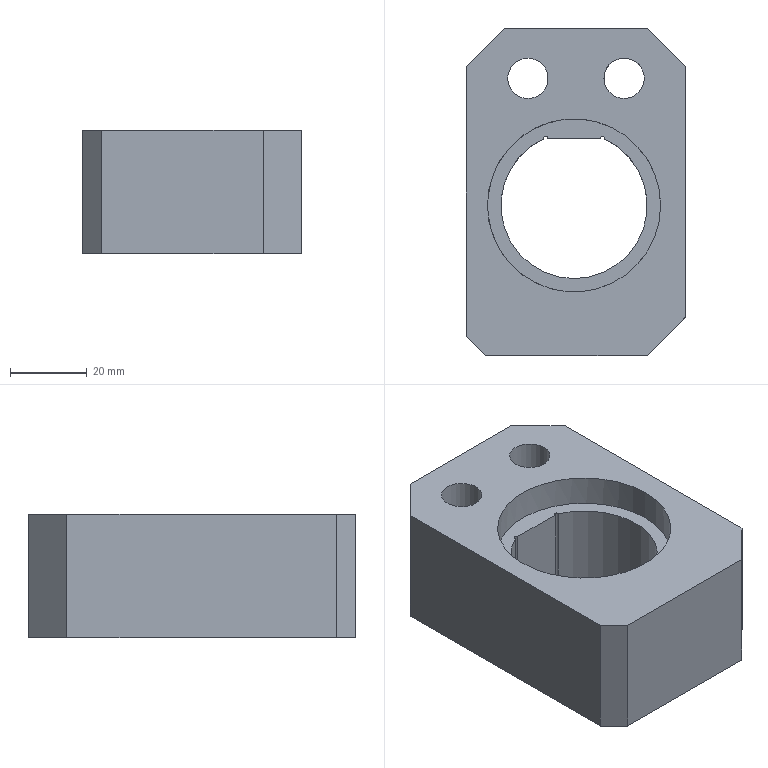Part | STEP file | lll_id3522_x_t | 1 solid | 23 faces | box 57 x 85 x 32 mm | volume 99919 mm3 | plane 14 | cylinder 9 | commonest cylinder face diameters 1 x2 10.5 x2 17 x2 38 x2 45 x1
STEP:
#1=CARTESIAN_POINT('',(3442.,57.,84.5));
#2=VERTEX_POINT('',#1);
#3=CARTESIAN_POINT('',(3419.5,57.,84.5));
#4=DIRECTION('',(0.,0.,-1.));
#5=DIRECTION('',(1.,0.,0.));
#6=AXIS2_PLACEMENT_3D('',#3,#4,#5);
#7=CIRCLE('',#6,22.5);
#8=EDGE_CURVE('',#2,#2,#7,.T.);
#9=ORIENTED_EDGE('',*,*,#8,.F.);
#10=EDGE_LOOP('',(#9));
#11=FACE_BOUND('',#10,.T.);
#12=CARTESIAN_POINT('',(3427.357,74.299,84.5));
#13=VERTEX_POINT('',#12);
#14=CARTESIAN_POINT('',(3426.399,74.5,84.5));
#15=VERTEX_POINT('',#14);
#16=CARTESIAN_POINT('',(3426.899,74.5,84.5));
#17=DIRECTION('',(0.,0.,1.));
#18=DIRECTION('',(-1.,0.,0.));
#19=AXIS2_PLACEMENT_3D('',#16,#17,#18);
#20=CIRCLE('',#19,0.5);
#21=EDGE_CURVE('',#13,#15,#20,.T.);
#22=ORIENTED_EDGE('',*,*,#21,.F.);
#23=CARTESIAN_POINT('',(3419.5,38.,84.5));
#24=VERTEX_POINT('',#23);
#25=CARTESIAN_POINT('',(3419.5,57.,84.5));
#26=DIRECTION('',(0.,0.,1.));
#27=DIRECTION('',(0.,-1.,0.));
#28=AXIS2_PLACEMENT_3D('',#25,#26,#27);
#29=CIRCLE('',#28,19.);
#30=EDGE_CURVE('',#24,#13,#29,.T.);
#31=ORIENTED_EDGE('',*,*,#30,.F.);
#32=CARTESIAN_POINT('',(3411.643,74.299,84.5));
#33=VERTEX_POINT('',#32);
#34=CARTESIAN_POINT('',(3419.5,57.,84.5));
#35=DIRECTION('',(0.,0.,1.));
#36=DIRECTION('',(0.,-1.,0.));
#37=AXIS2_PLACEMENT_3D('',#34,#35,#36);
#38=CIRCLE('',#37,19.);
#39=EDGE_CURVE('',#33,#24,#38,.T.);
#40=ORIENTED_EDGE('',*,*,#39,.F.);
#41=CARTESIAN_POINT('',(3412.601,74.5,84.5));
#42=VERTEX_POINT('',#41);
#43=CARTESIAN_POINT('',(3412.101,74.5,84.5));
#44=DIRECTION('',(0.,0.,-1.));
#45=DIRECTION('',(1.,0.,0.));
#46=AXIS2_PLACEMENT_3D('',#43,#44,#45);
#47=CIRCLE('',#46,0.5);
#48=EDGE_CURVE('',#33,#42,#47,.T.);
#49=ORIENTED_EDGE('',*,*,#48,.T.);
#50=CARTESIAN_POINT('',(3439.75,74.5,84.5));
#51=DIRECTION('',(1.,0.,0.));
#52=VECTOR('',#51,1.);
#53=LINE('',#50,#52);
#54=EDGE_CURVE('',#42,#15,#53,.T.);
#55=ORIENTED_EDGE('',*,*,#54,.T.);
#56=EDGE_LOOP('',(#22,#31,#40,#49,#55));
#57=FACE_BOUND('',#56,.T.);
#58=CARTESIAN_POINT('',(3439.75,57.,84.5));
#59=DIRECTION('',(0.,0.,-1.));
#60=DIRECTION('',(1.,0.,0.));
#61=AXIS2_PLACEMENT_3D('',#58,#59,#60);
#62=PLANE('',#61);
#63=ADVANCED_FACE('',(#11,#57),#62,.F.);
#64=CARTESIAN_POINT('',(3407.5,84.75,77.5));
#65=VERTEX_POINT('',#64);
#66=CARTESIAN_POINT('',(3407.5,90.,77.5));
#67=DIRECTION('',(0.,0.,1.));
#68=DIRECTION('',(0.,-1.,0.));
#69=AXIS2_PLACEMENT_3D('',#66,#67,#68);
#70=CIRCLE('',#69,5.25);
#71=EDGE_CURVE('',#65,#65,#70,.T.);
#72=ORIENTED_EDGE('',*,*,#71,.T.);
#73=EDGE_LOOP('',(#72));
#74=FACE_BOUND('',#73,.T.);
#75=CARTESIAN_POINT('',(3407.5,81.5,77.5));
#76=VERTEX_POINT('',#75);
#77=CARTESIAN_POINT('',(3407.5,90.,77.5));
#78=DIRECTION('',(0.,0.,1.));
#79=DIRECTION('',(0.,-1.,0.));
#80=AXIS2_PLACEMENT_3D('',#77,#78,#79);
#81=CIRCLE('',#80,8.5);
#82=EDGE_CURVE('',#76,#76,#81,.T.);
#83=ORIENTED_EDGE('',*,*,#82,.F.);
#84=EDGE_LOOP('',(#83));
#85=FACE_BOUND('',#84,.T.);
#86=CARTESIAN_POINT('',(3407.5,90.,77.5));
#87=DIRECTION('',(0.,0.,1.));
#88=DIRECTION('',(-1.,0.,0.));
#89=AXIS2_PLACEMENT_3D('',#86,#87,#88);
#90=PLANE('',#89);
#91=ADVANCED_FACE('',(#74,#85),#90,.F.);
#92=ORIENTED_EDGE('',*,*,#82,.T.);
#93=EDGE_LOOP('',(#92));
#94=FACE_BOUND('',#93,.T.);
#95=CARTESIAN_POINT('',(3407.5,81.5,60.5));
#96=VERTEX_POINT('',#95);
#97=CARTESIAN_POINT('',(3407.5,90.,60.5));
#98=DIRECTION('',(0.,0.,-1.));
#99=DIRECTION('',(0.,-1.,0.));
#100=AXIS2_PLACEMENT_3D('',#97,#98,#99);
#101=CIRCLE('',#100,8.5);
#102=EDGE_CURVE('',#96,#96,#101,.T.);
#103=ORIENTED_EDGE('',*,*,#102,.T.);
#104=EDGE_LOOP('',(#103));
#105=FACE_BOUND('',#104,.T.);
#106=CARTESIAN_POINT('',(3407.5,90.,60.5));
#107=DIRECTION('',(0.,0.,1.));
#108=DIRECTION('',(-1.,0.,0.));
#109=AXIS2_PLACEMENT_3D('',#106,#107,#108);
#110=CYLINDRICAL_SURFACE('',#109,8.5);
#111=ADVANCED_FACE('',(#94,#105),#110,.F.);
#112=CARTESIAN_POINT('',(3401.5,103.,92.5));
#113=VERTEX_POINT('',#112);
#114=CARTESIAN_POINT('',(3391.5,93.,92.5));
#115=VERTEX_POINT('',#114);
#116=CARTESIAN_POINT('',(3369.293,70.793,92.5));
#117=DIRECTION('',(-0.7071,-0.7071,0.));
#118=VECTOR('',#117,1.);
#119=LINE('',#116,#118);
#120=EDGE_CURVE('',#113,#115,#119,.T.);
#121=ORIENTED_EDGE('',*,*,#120,.F.);
#122=CARTESIAN_POINT('',(3401.5,103.,60.5));
#123=VERTEX_POINT('',#122);
#124=CARTESIAN_POINT('',(3401.5,103.,-8.5));
#125=DIRECTION('',(0.,0.,1.));
#126=VECTOR('',#125,1.);
#127=LINE('',#124,#126);
#128=EDGE_CURVE('',#123,#113,#127,.T.);
#129=ORIENTED_EDGE('',*,*,#128,.F.);
#130=CARTESIAN_POINT('',(3391.5,93.,60.5));
#131=VERTEX_POINT('',#130);
#132=CARTESIAN_POINT('',(3369.293,70.793,60.5));
#133=DIRECTION('',(0.7071,0.7071,0.));
#134=VECTOR('',#133,1.);
#135=LINE('',#132,#134);
#136=EDGE_CURVE('',#131,#123,#135,.T.);
#137=ORIENTED_EDGE('',*,*,#136,.F.);
#138=CARTESIAN_POINT('',(3391.5,93.,-8.5));
#139=DIRECTION('',(0.,0.,-1.));
#140=VECTOR('',#139,1.);
#141=LINE('',#138,#140);
#142=EDGE_CURVE('',#115,#131,#141,.T.);
#143=ORIENTED_EDGE('',*,*,#142,.F.);
#144=EDGE_LOOP('',(#121,#129,#137,#143));
#145=FACE_OUTER_BOUND('',#144,.T.);
#146=CARTESIAN_POINT('',(3391.5,93.,-8.5));
#147=DIRECTION('',(0.7071,-0.7071,0.));
#148=DIRECTION('',(0.,0.,-1.));
#149=AXIS2_PLACEMENT_3D('',#146,#147,#148);
#150=PLANE('',#149);
#151=ADVANCED_FACE('',(#145),#150,.F.);
#152=CARTESIAN_POINT('',(3438.5,103.,60.5));
#153=VERTEX_POINT('',#152);
#154=CARTESIAN_POINT('',(3356.31,103.,60.5));
#155=DIRECTION('',(1.,0.,0.));
#156=VECTOR('',#155,1.);
#157=LINE('',#154,#156);
#158=EDGE_CURVE('',#123,#153,#157,.T.);
#159=ORIENTED_EDGE('',*,*,#158,.F.);
#160=ORIENTED_EDGE('',*,*,#128,.T.);
#161=CARTESIAN_POINT('',(3438.5,103.,92.5));
#162=VERTEX_POINT('',#161);
#163=CARTESIAN_POINT('',(3351.36,103.,92.5));
#164=DIRECTION('',(-1.,0.,0.));
#165=VECTOR('',#164,1.);
#166=LINE('',#163,#165);
#167=EDGE_CURVE('',#162,#113,#166,.T.);
#168=ORIENTED_EDGE('',*,*,#167,.F.);
#169=CARTESIAN_POINT('',(3438.5,103.,-8.5));
#170=DIRECTION('',(0.,0.,-1.));
#171=VECTOR('',#170,1.);
#172=LINE('',#169,#171);
#173=EDGE_CURVE('',#162,#153,#172,.T.);
#174=ORIENTED_EDGE('',*,*,#173,.T.);
#175=EDGE_LOOP('',(#159,#160,#168,#174));
#176=FACE_OUTER_BOUND('',#175,.T.);
#177=CARTESIAN_POINT('',(3419.5,103.,-8.5));
#178=DIRECTION('',(0.,1.,0.));
#179=DIRECTION('',(0.,0.,1.));
#180=AXIS2_PLACEMENT_3D('',#177,#178,#179);
#181=PLANE('',#180);
#182=ADVANCED_FACE('',(#176),#181,.T.);
#183=CARTESIAN_POINT('',(3448.5,93.,60.5));
#184=VERTEX_POINT('',#183);
#185=CARTESIAN_POINT('',(3408.017,133.483,60.5));
#186=DIRECTION('',(0.7071,-0.7071,0.));
#187=VECTOR('',#186,1.);
#188=LINE('',#185,#187);
#189=EDGE_CURVE('',#153,#184,#188,.T.);
#190=ORIENTED_EDGE('',*,*,#189,.F.);
#191=ORIENTED_EDGE('',*,*,#173,.F.);
#192=CARTESIAN_POINT('',(3448.5,93.,92.5));
#193=VERTEX_POINT('',#192);
#194=CARTESIAN_POINT('',(3403.067,138.433,92.5));
#195=DIRECTION('',(-0.7071,0.7071,0.));
#196=VECTOR('',#195,1.);
#197=LINE('',#194,#196);
#198=EDGE_CURVE('',#193,#162,#197,.T.);
#199=ORIENTED_EDGE('',*,*,#198,.F.);
#200=CARTESIAN_POINT('',(3448.5,93.,-8.5));
#201=DIRECTION('',(0.,0.,1.));
#202=VECTOR('',#201,1.);
#203=LINE('',#200,#202);
#204=EDGE_CURVE('',#184,#193,#203,.T.);
#205=ORIENTED_EDGE('',*,*,#204,.F.);
#206=EDGE_LOOP('',(#190,#191,#199,#205));
#207=FACE_OUTER_BOUND('',#206,.T.);
#208=CARTESIAN_POINT('',(3448.5,93.,-8.5));
#209=DIRECTION('',(-0.7071,-0.7071,0.));
#210=DIRECTION('',(0.,0.,1.));
#211=AXIS2_PLACEMENT_3D('',#208,#209,#210);
#212=PLANE('',#211);
#213=ADVANCED_FACE('',(#207),#212,.F.);
#214=CARTESIAN_POINT('',(3448.5,28.,60.5));
#215=VERTEX_POINT('',#214);
#216=CARTESIAN_POINT('',(3448.5,83.276,60.5));
#217=DIRECTION('',(0.,-1.,0.));
#218=VECTOR('',#217,1.);
#219=LINE('',#216,#218);
#220=EDGE_CURVE('',#184,#215,#219,.T.);
#221=ORIENTED_EDGE('',*,*,#220,.F.);
#222=ORIENTED_EDGE('',*,*,#204,.T.);
#223=CARTESIAN_POINT('',(3448.5,28.,92.5));
#224=VERTEX_POINT('',#223);
#225=CARTESIAN_POINT('',(3448.5,88.226,92.5));
#226=DIRECTION('',(0.,1.,0.));
#227=VECTOR('',#226,1.);
#228=LINE('',#225,#227);
#229=EDGE_CURVE('',#224,#193,#228,.T.);
#230=ORIENTED_EDGE('',*,*,#229,.F.);
#231=CARTESIAN_POINT('',(3448.5,28.,-8.5));
#232=DIRECTION('',(0.,0.,-1.));
#233=VECTOR('',#232,1.);
#234=LINE('',#231,#233);
#235=EDGE_CURVE('',#224,#215,#234,.T.);
#236=ORIENTED_EDGE('',*,*,#235,.T.);
#237=EDGE_LOOP('',(#221,#222,#230,#236));
#238=FACE_OUTER_BOUND('',#237,.T.);
#239=CARTESIAN_POINT('',(3448.5,52.05,-8.5));
#240=DIRECTION('',(1.,0.,0.));
#241=DIRECTION('',(0.,0.,1.));
#242=AXIS2_PLACEMENT_3D('',#239,#240,#241);
#243=PLANE('',#242);
#244=ADVANCED_FACE('',(#238),#243,.T.);
#245=CARTESIAN_POINT('',(3438.5,18.,92.5));
#246=VERTEX_POINT('',#245);
#247=CARTESIAN_POINT('',(3424.793,4.293,92.5));
#248=DIRECTION('',(0.7071,0.7071,0.));
#249=VECTOR('',#248,1.);
#250=LINE('',#247,#249);
#251=EDGE_CURVE('',#246,#224,#250,.T.);
#252=ORIENTED_EDGE('',*,*,#251,.F.);
#253=CARTESIAN_POINT('',(3438.5,18.,60.5));
#254=VERTEX_POINT('',#253);
#255=CARTESIAN_POINT('',(3438.5,18.,-8.5));
#256=DIRECTION('',(0.,0.,1.));
#257=VECTOR('',#256,1.);
#258=LINE('',#255,#257);
#259=EDGE_CURVE('',#254,#246,#258,.T.);
#260=ORIENTED_EDGE('',*,*,#259,.F.);
#261=CARTESIAN_POINT('',(3424.793,4.293,60.5));
#262=DIRECTION('',(-0.7071,-0.7071,0.));
#263=VECTOR('',#262,1.);
#264=LINE('',#261,#263);
#265=EDGE_CURVE('',#215,#254,#264,.T.);
#266=ORIENTED_EDGE('',*,*,#265,.F.);
#267=ORIENTED_EDGE('',*,*,#235,.F.);
#268=EDGE_LOOP('',(#252,#260,#266,#267));
#269=FACE_OUTER_BOUND('',#268,.T.);
#270=CARTESIAN_POINT('',(3448.5,28.,-8.5));
#271=DIRECTION('',(-0.7071,0.7071,0.));
#272=DIRECTION('',(0.,0.,-1.));
#273=AXIS2_PLACEMENT_3D('',#270,#271,#272);
#274=PLANE('',#273);
#275=ADVANCED_FACE('',(#269),#274,.F.);
#276=CARTESIAN_POINT('',(3396.5,18.,92.5));
#277=VERTEX_POINT('',#276);
#278=CARTESIAN_POINT('',(3351.36,18.,92.5));
#279=DIRECTION('',(1.,0.,0.));
#280=VECTOR('',#279,1.);
#281=LINE('',#278,#280);
#282=EDGE_CURVE('',#277,#246,#281,.T.);
#283=ORIENTED_EDGE('',*,*,#282,.F.);
#284=CARTESIAN_POINT('',(3396.5,18.,60.5));
#285=VERTEX_POINT('',#284);
#286=CARTESIAN_POINT('',(3396.5,18.,-8.5));
#287=DIRECTION('',(0.,0.,-1.));
#288=VECTOR('',#287,1.);
#289=LINE('',#286,#288);
#290=EDGE_CURVE('',#277,#285,#289,.T.);
#291=ORIENTED_EDGE('',*,*,#290,.T.);
#292=CARTESIAN_POINT('',(3356.31,18.,60.5));
#293=DIRECTION('',(-1.,0.,0.));
#294=VECTOR('',#293,1.);
#295=LINE('',#292,#294);
#296=EDGE_CURVE('',#254,#285,#295,.T.);
#297=ORIENTED_EDGE('',*,*,#296,.F.);
#298=ORIENTED_EDGE('',*,*,#259,.T.);
#299=EDGE_LOOP('',(#283,#291,#297,#298));
#300=FACE_OUTER_BOUND('',#299,.T.);
#301=CARTESIAN_POINT('',(3419.5,18.,-8.5));
#302=DIRECTION('',(0.,-1.,0.));
#303=DIRECTION('',(0.,0.,-1.));
#304=AXIS2_PLACEMENT_3D('',#301,#302,#303);
#305=PLANE('',#304);
#306=ADVANCED_FACE('',(#300),#305,.T.);
#307=CARTESIAN_POINT('',(3391.5,23.,92.5));
#308=VERTEX_POINT('',#307);
#309=CARTESIAN_POINT('',(3344.567,69.933,92.5));
#310=DIRECTION('',(0.7071,-0.7071,0.));
#311=VECTOR('',#310,1.);
#312=LINE('',#309,#311);
#313=EDGE_CURVE('',#308,#277,#312,.T.);
#314=ORIENTED_EDGE('',*,*,#313,.F.);
#315=CARTESIAN_POINT('',(3391.5,23.,60.5));
#316=VERTEX_POINT('',#315);
#317=CARTESIAN_POINT('',(3391.5,23.,-8.5));
#318=DIRECTION('',(0.,0.,1.));
#319=VECTOR('',#318,1.);
#320=LINE('',#317,#319);
#321=EDGE_CURVE('',#316,#308,#320,.T.);
#322=ORIENTED_EDGE('',*,*,#321,.F.);
#323=CARTESIAN_POINT('',(3349.517,64.983,60.5));
#324=DIRECTION('',(-0.7071,0.7071,0.));
#325=VECTOR('',#324,1.);
#326=LINE('',#323,#325);
#327=EDGE_CURVE('',#285,#316,#326,.T.);
#328=ORIENTED_EDGE('',*,*,#327,.F.);
#329=ORIENTED_EDGE('',*,*,#290,.F.);
#330=EDGE_LOOP('',(#314,#322,#328,#329));
#331=FACE_OUTER_BOUND('',#330,.T.);
#332=CARTESIAN_POINT('',(3396.5,18.,-8.5));
#333=DIRECTION('',(0.7071,0.7071,0.));
#334=DIRECTION('',(0.,0.,-1.));
#335=AXIS2_PLACEMENT_3D('',#332,#333,#334);
#336=PLANE('',#335);
#337=ADVANCED_FACE('',(#331),#336,.F.);
#338=CARTESIAN_POINT('',(3391.5,83.276,60.5));
#339=DIRECTION('',(0.,1.,0.));
#340=VECTOR('',#339,1.);
#341=LINE('',#338,#340);
#342=EDGE_CURVE('',#316,#131,#341,.T.);
#343=ORIENTED_EDGE('',*,*,#342,.F.);
#344=ORIENTED_EDGE('',*,*,#321,.T.);
#345=CARTESIAN_POINT('',(3391.5,88.226,92.5));
#346=DIRECTION('',(0.,-1.,0.));
#347=VECTOR('',#346,1.);
#348=LINE('',#345,#347);
#349=EDGE_CURVE('',#115,#308,#348,.T.);
#350=ORIENTED_EDGE('',*,*,#349,.F.);
#351=ORIENTED_EDGE('',*,*,#142,.T.);
#352=EDGE_LOOP('',(#343,#344,#350,#351));
#353=FACE_OUTER_BOUND('',#352,.T.);
#354=CARTESIAN_POINT('',(3391.5,57.,-8.5));
#355=DIRECTION('',(-1.,0.,0.));
#356=DIRECTION('',(0.,0.,-1.));
#357=AXIS2_PLACEMENT_3D('',#354,#355,#356);
#358=PLANE('',#357);
#359=ADVANCED_FACE('',(#353),#358,.T.);
#360=CARTESIAN_POINT('',(3407.5,84.75,92.5));
#361=VERTEX_POINT('',#360);
#362=CARTESIAN_POINT('',(3407.5,90.,92.5));
#363=DIRECTION('',(0.,0.,-1.));
#364=DIRECTION('',(0.,-1.,0.));
#365=AXIS2_PLACEMENT_3D('',#362,#363,#364);
#366=CIRCLE('',#365,5.25);
#367=EDGE_CURVE('',#361,#361,#366,.T.);
#368=ORIENTED_EDGE('',*,*,#367,.F.);
#369=EDGE_LOOP('',(#368));
#370=FACE_BOUND('',#369,.T.);
#371=ORIENTED_EDGE('',*,*,#71,.F.);
#372=EDGE_LOOP('',(#371));
#373=FACE_BOUND('',#372,.T.);
#374=CARTESIAN_POINT('',(3407.5,90.,160.5));
#375=DIRECTION('',(0.,0.,1.));
#376=DIRECTION('',(-1.,0.,0.));
#377=AXIS2_PLACEMENT_3D('',#374,#375,#376);
#378=CYLINDRICAL_SURFACE('',#377,5.25);
#379=ADVANCED_FACE('',(#370,#373),#378,.F.);
#380=ORIENTED_EDGE('',*,*,#8,.T.);
#381=EDGE_LOOP('',(#380));
#382=FACE_BOUND('',#381,.T.);
#383=CARTESIAN_POINT('',(3397.,57.,92.5));
#384=VERTEX_POINT('',#383);
#385=CARTESIAN_POINT('',(3419.5,57.,92.5));
#386=DIRECTION('',(0.,0.,1.));
#387=DIRECTION('',(-1.,0.,0.));
#388=AXIS2_PLACEMENT_3D('',#385,#386,#387);
#389=CIRCLE('',#388,22.5);
#390=EDGE_CURVE('',#384,#384,#389,.T.);
#391=ORIENTED_EDGE('',*,*,#390,.T.);
#392=EDGE_LOOP('',(#391));
#393=FACE_BOUND('',#392,.T.);
#394=CARTESIAN_POINT('',(3419.5,57.,88.5));
#395=DIRECTION('',(0.,0.,-1.));
#396=DIRECTION('',(0.,1.,0.));
#397=AXIS2_PLACEMENT_3D('',#394,#395,#396);
#398=CYLINDRICAL_SURFACE('',#397,22.5);
#399=ADVANCED_FACE('',(#382,#393),#398,.F.);
#400=CARTESIAN_POINT('',(3437.75,90.,92.5));
#401=VERTEX_POINT('',#400);
#402=CARTESIAN_POINT('',(3432.5,90.,92.5));
#403=DIRECTION('',(0.,0.,1.));
#404=DIRECTION('',(1.,0.,0.));
#405=AXIS2_PLACEMENT_3D('',#402,#403,#404);
#406=CIRCLE('',#405,5.25);
#407=EDGE_CURVE('',#401,#401,#406,.T.);
#408=ORIENTED_EDGE('',*,*,#407,.F.);
#409=EDGE_LOOP('',(#408));
#410=FACE_BOUND('',#409,.T.);
#411=ORIENTED_EDGE('',*,*,#390,.F.);
#412=EDGE_LOOP('',(#411));
#413=FACE_BOUND('',#412,.T.);
#414=ORIENTED_EDGE('',*,*,#367,.T.);
#415=EDGE_LOOP('',(#414));
#416=FACE_BOUND('',#415,.T.);
#417=ORIENTED_EDGE('',*,*,#349,.T.);
#418=ORIENTED_EDGE('',*,*,#313,.T.);
#419=ORIENTED_EDGE('',*,*,#282,.T.);
#420=ORIENTED_EDGE('',*,*,#251,.T.);
#421=ORIENTED_EDGE('',*,*,#229,.T.);
#422=ORIENTED_EDGE('',*,*,#198,.T.);
#423=ORIENTED_EDGE('',*,*,#167,.T.);
#424=ORIENTED_EDGE('',*,*,#120,.T.);
#425=EDGE_LOOP('',(#417,#418,#419,#420,#421,#422,#423,#424));
#426=FACE_BOUND('',#425,.T.);
#427=CARTESIAN_POINT('',(3351.36,88.226,92.5));
#428=DIRECTION('',(0.,0.,1.));
#429=DIRECTION('',(-1.,0.,0.));
#430=AXIS2_PLACEMENT_3D('',#427,#428,#429);
#431=PLANE('',#430);
#432=ADVANCED_FACE('',(#410,#413,#416,#426),#431,.T.);
#433=CARTESIAN_POINT('',(3426.399,74.5,60.5));
#434=VERTEX_POINT('',#433);
#435=CARTESIAN_POINT('',(3427.357,74.299,60.5));
#436=VERTEX_POINT('',#435);
#437=CARTESIAN_POINT('',(3426.899,74.5,60.5));
#438=DIRECTION('',(0.,0.,-1.));
#439=DIRECTION('',(1.,0.,0.));
#440=AXIS2_PLACEMENT_3D('',#437,#438,#439);
#441=CIRCLE('',#440,0.5);
#442=EDGE_CURVE('',#434,#436,#441,.T.);
#443=ORIENTED_EDGE('',*,*,#442,.F.);
#444=CARTESIAN_POINT('',(3412.601,74.5,60.5));
#445=VERTEX_POINT('',#444);
#446=CARTESIAN_POINT('',(3356.31,74.5,60.5));
#447=DIRECTION('',(1.,0.,0.));
#448=VECTOR('',#447,1.);
#449=LINE('',#446,#448);
#450=EDGE_CURVE('',#445,#434,#449,.T.);
#451=ORIENTED_EDGE('',*,*,#450,.F.);
#452=CARTESIAN_POINT('',(3411.643,74.299,60.5));
#453=VERTEX_POINT('',#452);
#454=CARTESIAN_POINT('',(3412.101,74.5,60.5));
#455=DIRECTION('',(0.,0.,-1.));
#456=DIRECTION('',(1.,0.,0.));
#457=AXIS2_PLACEMENT_3D('',#454,#455,#456);
#458=CIRCLE('',#457,0.5);
#459=EDGE_CURVE('',#453,#445,#458,.T.);
#460=ORIENTED_EDGE('',*,*,#459,.F.);
#461=CARTESIAN_POINT('',(3419.5,38.,60.5));
#462=VERTEX_POINT('',#461);
#463=CARTESIAN_POINT('',(3419.5,57.,60.5));
#464=DIRECTION('',(0.,0.,-1.));
#465=DIRECTION('',(1.,0.,0.));
#466=AXIS2_PLACEMENT_3D('',#463,#464,#465);
#467=CIRCLE('',#466,19.);
#468=EDGE_CURVE('',#462,#453,#467,.T.);
#469=ORIENTED_EDGE('',*,*,#468,.F.);
#470=CARTESIAN_POINT('',(3419.5,57.,60.5));
#471=DIRECTION('',(0.,0.,-1.));
#472=DIRECTION('',(1.,0.,0.));
#473=AXIS2_PLACEMENT_3D('',#470,#471,#472);
#474=CIRCLE('',#473,19.);
#475=EDGE_CURVE('',#436,#462,#474,.T.);
#476=ORIENTED_EDGE('',*,*,#475,.F.);
#477=EDGE_LOOP('',(#443,#451,#460,#469,#476));
#478=FACE_BOUND('',#477,.T.);
#479=CARTESIAN_POINT('',(3441.,90.,60.5));
#480=VERTEX_POINT('',#479);
#481=CARTESIAN_POINT('',(3432.5,90.,60.5));
#482=DIRECTION('',(0.,0.,-1.));
#483=DIRECTION('',(1.,0.,0.));
#484=AXIS2_PLACEMENT_3D('',#481,#482,#483);
#485=CIRCLE('',#484,8.5);
#486=EDGE_CURVE('',#480,#480,#485,.T.);
#487=ORIENTED_EDGE('',*,*,#486,.F.);
#488=EDGE_LOOP('',(#487));
#489=FACE_BOUND('',#488,.T.);
#490=ORIENTED_EDGE('',*,*,#296,.T.);
#491=ORIENTED_EDGE('',*,*,#327,.T.);
#492=ORIENTED_EDGE('',*,*,#342,.T.);
#493=ORIENTED_EDGE('',*,*,#136,.T.);
#494=ORIENTED_EDGE('',*,*,#158,.T.);
#495=ORIENTED_EDGE('',*,*,#189,.T.);
#496=ORIENTED_EDGE('',*,*,#220,.T.);
#497=ORIENTED_EDGE('',*,*,#265,.T.);
#498=EDGE_LOOP('',(#490,#491,#492,#493,#494,#495,#496,#497));
#499=FACE_BOUND('',#498,.T.);
#500=ORIENTED_EDGE('',*,*,#102,.F.);
#501=EDGE_LOOP('',(#500));
#502=FACE_BOUND('',#501,.T.);
#503=CARTESIAN_POINT('',(3356.31,83.276,60.5));
#504=DIRECTION('',(0.,0.,1.));
#505=DIRECTION('',(-1.,0.,0.));
#506=AXIS2_PLACEMENT_3D('',#503,#504,#505);
#507=PLANE('',#506);
#508=ADVANCED_FACE('',(#478,#489,#499,#502),#507,.F.);
#509=CARTESIAN_POINT('',(3432.5,84.75,77.5));
#510=VERTEX_POINT('',#509);
#511=CARTESIAN_POINT('',(3432.5,90.,77.5));
#512=DIRECTION('',(0.,0.,1.));
#513=DIRECTION('',(0.,-1.,0.));
#514=AXIS2_PLACEMENT_3D('',#511,#512,#513);
#515=CIRCLE('',#514,5.25);
#516=EDGE_CURVE('',#510,#510,#515,.T.);
#517=ORIENTED_EDGE('',*,*,#516,.T.);
#518=EDGE_LOOP('',(#517));
#519=FACE_BOUND('',#518,.T.);
#520=CARTESIAN_POINT('',(3432.5,81.5,77.5));
#521=VERTEX_POINT('',#520);
#522=CARTESIAN_POINT('',(3432.5,90.,77.5));
#523=DIRECTION('',(0.,0.,1.));
#524=DIRECTION('',(0.,-1.,0.));
#525=AXIS2_PLACEMENT_3D('',#522,#523,#524);
#526=CIRCLE('',#525,8.5);
#527=EDGE_CURVE('',#521,#521,#526,.T.);
#528=ORIENTED_EDGE('',*,*,#527,.F.);
#529=EDGE_LOOP('',(#528));
#530=FACE_BOUND('',#529,.T.);
#531=CARTESIAN_POINT('',(3432.5,90.,77.5));
#532=DIRECTION('',(0.,0.,1.));
#533=DIRECTION('',(1.,0.,0.));
#534=AXIS2_PLACEMENT_3D('',#531,#532,#533);
#535=PLANE('',#534);
#536=ADVANCED_FACE('',(#519,#530),#535,.F.);
#537=ORIENTED_EDGE('',*,*,#407,.T.);
#538=EDGE_LOOP('',(#537));
#539=FACE_BOUND('',#538,.T.);
#540=ORIENTED_EDGE('',*,*,#516,.F.);
#541=EDGE_LOOP('',(#540));
#542=FACE_BOUND('',#541,.T.);
#543=CARTESIAN_POINT('',(3432.5,90.,160.5));
#544=DIRECTION('',(0.,0.,1.));
#545=DIRECTION('',(1.,0.,0.));
#546=AXIS2_PLACEMENT_3D('',#543,#544,#545);
#547=CYLINDRICAL_SURFACE('',#546,5.25);
#548=ADVANCED_FACE('',(#539,#542),#547,.F.);
#549=ORIENTED_EDGE('',*,*,#527,.T.);
#550=EDGE_LOOP('',(#549));
#551=FACE_BOUND('',#550,.T.);
#552=ORIENTED_EDGE('',*,*,#486,.T.);
#553=EDGE_LOOP('',(#552));
#554=FACE_BOUND('',#553,.T.);
#555=CARTESIAN_POINT('',(3432.5,90.,60.5));
#556=DIRECTION('',(0.,0.,1.));
#557=DIRECTION('',(1.,0.,0.));
#558=AXIS2_PLACEMENT_3D('',#555,#556,#557);
#559=CYLINDRICAL_SURFACE('',#558,8.5);
#560=ADVANCED_FACE('',(#551,#554),#559,.F.);
#561=ORIENTED_EDGE('',*,*,#450,.T.);
#562=CARTESIAN_POINT('',(3426.399,74.5,84.5));
#563=DIRECTION('',(0.,0.,1.));
#564=VECTOR('',#563,1.);
#565=LINE('',#562,#564);
#566=EDGE_CURVE('',#434,#15,#565,.T.);
#567=ORIENTED_EDGE('',*,*,#566,.T.);
#568=ORIENTED_EDGE('',*,*,#54,.F.);
#569=CARTESIAN_POINT('',(3412.601,74.5,84.5));
#570=DIRECTION('',(0.,0.,-1.));
#571=VECTOR('',#570,1.);
#572=LINE('',#569,#571);
#573=EDGE_CURVE('',#42,#445,#572,.T.);
#574=ORIENTED_EDGE('',*,*,#573,.T.);
#575=EDGE_LOOP('',(#561,#567,#568,#574));
#576=FACE_OUTER_BOUND('',#575,.T.);
#577=CARTESIAN_POINT('',(3419.5,74.5,61.5));
#578=DIRECTION('',(0.,1.,0.));
#579=DIRECTION('',(0.,0.,1.));
#580=AXIS2_PLACEMENT_3D('',#577,#578,#579);
#581=PLANE('',#580);
#582=ADVANCED_FACE('',(#576),#581,.F.);
#583=ORIENTED_EDGE('',*,*,#30,.T.);
#584=CARTESIAN_POINT('',(3427.357,74.299,67.));
#585=DIRECTION('',(0.,0.,-1.));
#586=VECTOR('',#585,1.);
#587=LINE('',#584,#586);
#588=EDGE_CURVE('',#13,#436,#587,.T.);
#589=ORIENTED_EDGE('',*,*,#588,.T.);
#590=ORIENTED_EDGE('',*,*,#475,.T.);
#591=CARTESIAN_POINT('',(3419.5,38.,38.5));
#592=DIRECTION('',(0.,0.,-1.));
#593=VECTOR('',#592,1.);
#594=LINE('',#591,#593);
#595=EDGE_CURVE('',#24,#462,#594,.T.);
#596=ORIENTED_EDGE('',*,*,#595,.F.);
#597=EDGE_LOOP('',(#583,#589,#590,#596));
#598=FACE_OUTER_BOUND('',#597,.T.);
#599=CARTESIAN_POINT('',(3419.5,57.,38.5));
#600=DIRECTION('',(0.,0.,-1.));
#601=DIRECTION('',(0.,1.,0.));
#602=AXIS2_PLACEMENT_3D('',#599,#600,#601);
#603=CYLINDRICAL_SURFACE('',#602,19.);
#604=ADVANCED_FACE('',(#598),#603,.F.);
#605=ORIENTED_EDGE('',*,*,#468,.T.);
#606=CARTESIAN_POINT('',(3411.643,74.299,67.));
#607=DIRECTION('',(0.,0.,1.));
#608=VECTOR('',#607,1.);
#609=LINE('',#606,#608);
#610=EDGE_CURVE('',#453,#33,#609,.T.);
#611=ORIENTED_EDGE('',*,*,#610,.T.);
#612=ORIENTED_EDGE('',*,*,#39,.T.);
#613=ORIENTED_EDGE('',*,*,#595,.T.);
#614=EDGE_LOOP('',(#605,#611,#612,#613));
#615=FACE_OUTER_BOUND('',#614,.T.);
#616=CARTESIAN_POINT('',(3419.5,57.,38.5));
#617=DIRECTION('',(0.,0.,-1.));
#618=DIRECTION('',(0.,1.,0.));
#619=AXIS2_PLACEMENT_3D('',#616,#617,#618);
#620=CYLINDRICAL_SURFACE('',#619,19.);
#621=ADVANCED_FACE('',(#615),#620,.F.);
#622=ORIENTED_EDGE('',*,*,#48,.F.);
#623=ORIENTED_EDGE('',*,*,#610,.F.);
#624=ORIENTED_EDGE('',*,*,#459,.T.);
#625=ORIENTED_EDGE('',*,*,#573,.F.);
#626=EDGE_LOOP('',(#622,#623,#624,#625));
#627=FACE_OUTER_BOUND('',#626,.T.);
#628=CARTESIAN_POINT('',(3412.101,74.5,84.5));
#629=DIRECTION('',(0.,0.,-1.));
#630=DIRECTION('',(1.,0.,0.));
#631=AXIS2_PLACEMENT_3D('',#628,#629,#630);
#632=CYLINDRICAL_SURFACE('',#631,0.5);
#633=ADVANCED_FACE('',(#627),#632,.F.);
#634=ORIENTED_EDGE('',*,*,#442,.T.);
#635=ORIENTED_EDGE('',*,*,#588,.F.);
#636=ORIENTED_EDGE('',*,*,#21,.T.);
#637=ORIENTED_EDGE('',*,*,#566,.F.);
#638=EDGE_LOOP('',(#634,#635,#636,#637));
#639=FACE_OUTER_BOUND('',#638,.T.);
#640=CARTESIAN_POINT('',(3426.899,74.5,84.5));
#641=DIRECTION('',(0.,0.,-1.));
#642=DIRECTION('',(-1.,0.,0.));
#643=AXIS2_PLACEMENT_3D('',#640,#641,#642);
#644=CYLINDRICAL_SURFACE('',#643,0.5);
#645=ADVANCED_FACE('',(#639),#644,.F.);
#646=CLOSED_SHELL('',(#63,#91,#111,#151,#182,#213,#244,#275,#306,#337,#359,#379,#399,#432,#508,#536,#548,#560,#582,#604,#621,#633,#645));
#647=MANIFOLD_SOLID_BREP('',#646);
#648=(LENGTH_UNIT()NAMED_UNIT(*)SI_UNIT(.MILLI.,.METRE.));
#649=UNCERTAINTY_MEASURE_WITH_UNIT(LENGTH_MEASURE(0.00002),#648,'','');
#650=(NAMED_UNIT(*)PLANE_ANGLE_UNIT()SI_UNIT($,.RADIAN.));
#651=PLANE_ANGLE_MEASURE_WITH_UNIT(PLANE_ANGLE_MEASURE(0.01745),#650);
#652=DIMENSIONAL_EXPONENTS(0.,0.,0.,0.,0.,0.,0.);
#653=(CONVERSION_BASED_UNIT('DEGREE',#651)NAMED_UNIT(#652)PLANE_ANGLE_UNIT());
#654=(NAMED_UNIT(*)SI_UNIT($,.STERADIAN.)SOLID_ANGLE_UNIT());
#655=(GEOMETRIC_REPRESENTATION_CONTEXT(3)GLOBAL_UNCERTAINTY_ASSIGNED_CONTEXT((#649))GLOBAL_UNIT_ASSIGNED_CONTEXT((#648,#653,#654))REPRESENTATION_CONTEXT('',''));
#656=ADVANCED_BREP_SHAPE_REPRESENTATION('',(#647),#655);